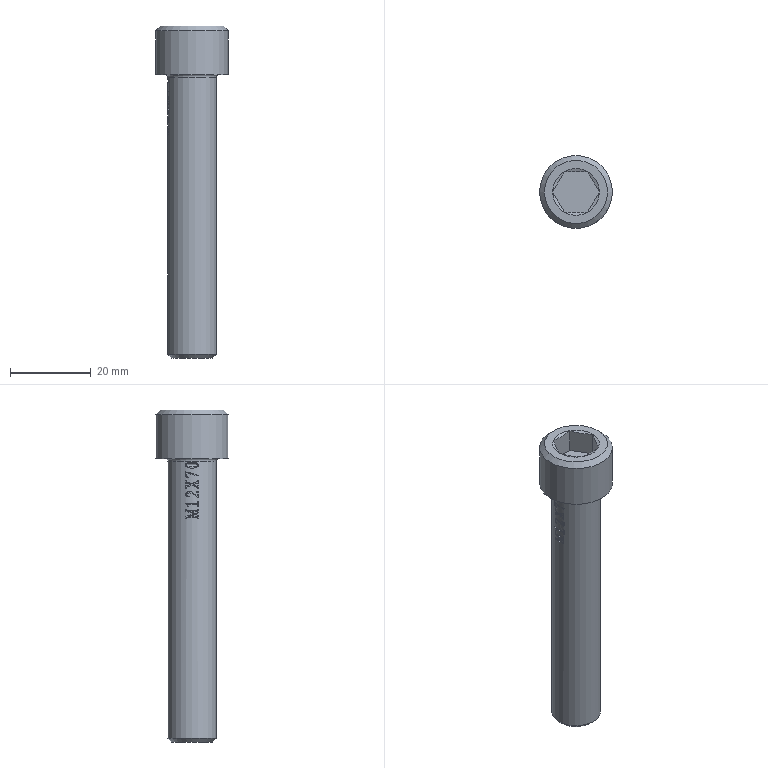Part | STEP file | solid 97 | 1 solid | 107 faces | box 18 x 18 x 82 mm | volume 10396 mm3 | plane 65 | other 27 | cylinder 6 | sphere 6 | cone 2 | torus 1 | commonest cylinder face diameters 12 x5 18 x1